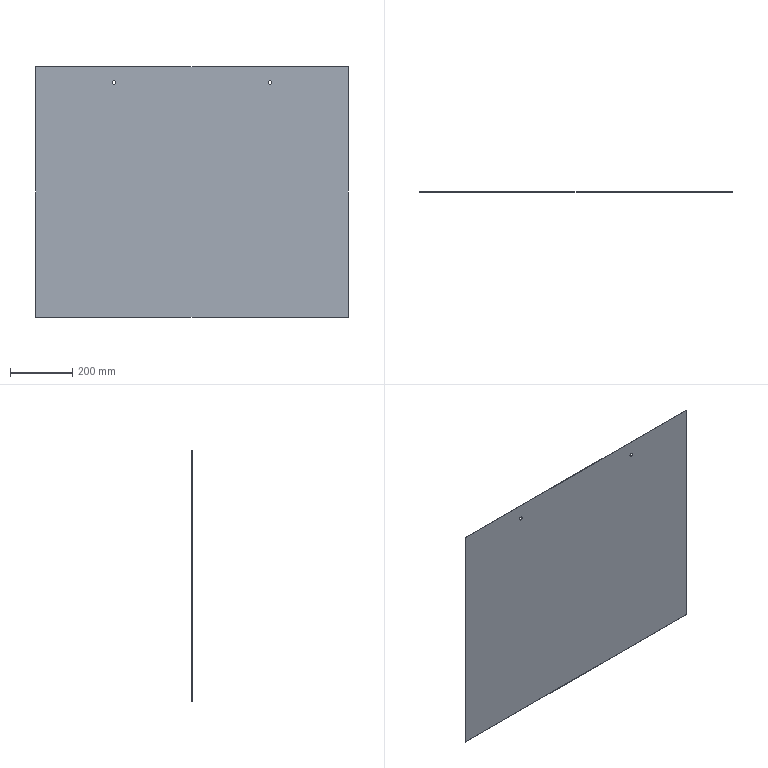Part | SolidWorks | features Extrusion 1, ICE 1 | 1 solid | 10 faces | box 1000 x 1 x 801 mm | volume 800810 mm3 | plane 6 | cylinder 4 | commonest cylinder face diameters 11 x4
STEP:
#1=CARTESIAN_POINT('',(-250.,0.,345.));
#2=VERTEX_POINT('',#1);
#3=CARTESIAN_POINT('',(-250.,0.,356.));
#4=VERTEX_POINT('',#3);
#5=CARTESIAN_POINT('',(-250.,0.,350.5));
#6=DIRECTION('',(0.,1.,0.));
#7=DIRECTION('',(0.,0.,1.));
#8=AXIS2_PLACEMENT_3D('',#5,#6,#7);
#9=CIRCLE('',#8,5.5);
#10=EDGE_CURVE('',#2,#4,#9,.T.);
#11=ORIENTED_EDGE('',*,*,#10,.F.);
#12=CARTESIAN_POINT('',(-250.,1.,345.));
#13=VERTEX_POINT('',#12);
#14=CARTESIAN_POINT('',(-250.,0.,345.));
#15=DIRECTION('',(0.,1.,0.));
#16=VECTOR('',#15,1000.);
#17=LINE('',#14,#16);
#18=EDGE_CURVE('',#2,#13,#17,.T.);
#19=ORIENTED_EDGE('',*,*,#18,.T.);
#20=CARTESIAN_POINT('',(-250.,1.,356.));
#21=VERTEX_POINT('',#20);
#22=CARTESIAN_POINT('',(-250.,1.,350.5));
#23=DIRECTION('',(0.,1.,0.));
#24=DIRECTION('',(0.,0.,1.));
#25=AXIS2_PLACEMENT_3D('',#22,#23,#24);
#26=CIRCLE('',#25,5.5);
#27=EDGE_CURVE('',#13,#21,#26,.T.);
#28=ORIENTED_EDGE('',*,*,#27,.T.);
#29=CARTESIAN_POINT('',(-250.,0.,356.));
#30=DIRECTION('',(0.,1.,0.));
#31=VECTOR('',#30,1000.);
#32=LINE('',#29,#31);
#33=EDGE_CURVE('',#4,#21,#32,.T.);
#34=ORIENTED_EDGE('',*,*,#33,.F.);
#35=EDGE_LOOP('',(#11,#19,#28,#34));
#36=FACE_OUTER_BOUND('',#35,.T.);
#37=CARTESIAN_POINT('',(-250.,0.,350.5));
#38=DIRECTION('',(0.,1.,0.));
#39=DIRECTION('',(0.,0.,1.));
#40=AXIS2_PLACEMENT_3D('',#37,#38,#39);
#41=CYLINDRICAL_SURFACE('',#40,5.5);
#42=ADVANCED_FACE('',(#36),#41,.F.);
#43=CARTESIAN_POINT('',(250.,0.,345.));
#44=VERTEX_POINT('',#43);
#45=CARTESIAN_POINT('',(250.,0.,356.));
#46=VERTEX_POINT('',#45);
#47=CARTESIAN_POINT('',(250.,0.,350.5));
#48=DIRECTION('',(0.,1.,0.));
#49=DIRECTION('',(0.,0.,1.));
#50=AXIS2_PLACEMENT_3D('',#47,#48,#49);
#51=CIRCLE('',#50,5.5);
#52=EDGE_CURVE('',#44,#46,#51,.T.);
#53=ORIENTED_EDGE('',*,*,#52,.F.);
#54=CARTESIAN_POINT('',(250.,1.,345.));
#55=VERTEX_POINT('',#54);
#56=CARTESIAN_POINT('',(250.,0.,345.));
#57=DIRECTION('',(0.,1.,0.));
#58=VECTOR('',#57,1000.);
#59=LINE('',#56,#58);
#60=EDGE_CURVE('',#44,#55,#59,.T.);
#61=ORIENTED_EDGE('',*,*,#60,.T.);
#62=CARTESIAN_POINT('',(250.,1.,356.));
#63=VERTEX_POINT('',#62);
#64=CARTESIAN_POINT('',(250.,1.,350.5));
#65=DIRECTION('',(0.,1.,0.));
#66=DIRECTION('',(0.,0.,1.));
#67=AXIS2_PLACEMENT_3D('',#64,#65,#66);
#68=CIRCLE('',#67,5.5);
#69=EDGE_CURVE('',#55,#63,#68,.T.);
#70=ORIENTED_EDGE('',*,*,#69,.T.);
#71=CARTESIAN_POINT('',(250.,0.,356.));
#72=DIRECTION('',(0.,1.,0.));
#73=VECTOR('',#72,1000.);
#74=LINE('',#71,#73);
#75=EDGE_CURVE('',#46,#63,#74,.T.);
#76=ORIENTED_EDGE('',*,*,#75,.F.);
#77=EDGE_LOOP('',(#53,#61,#70,#76));
#78=FACE_OUTER_BOUND('',#77,.T.);
#79=CARTESIAN_POINT('',(250.,0.,350.5));
#80=DIRECTION('',(0.,1.,0.));
#81=DIRECTION('',(0.,0.,1.));
#82=AXIS2_PLACEMENT_3D('',#79,#80,#81);
#83=CYLINDRICAL_SURFACE('',#82,5.5);
#84=ADVANCED_FACE('',(#78),#83,.F.);
#85=CARTESIAN_POINT('',(500.,0.,400.5));
#86=VERTEX_POINT('',#85);
#87=CARTESIAN_POINT('',(500.,0.,-400.5));
#88=VERTEX_POINT('',#87);
#89=CARTESIAN_POINT('',(500.,0.,400.5));
#90=DIRECTION('',(0.,0.,-1.));
#91=VECTOR('',#90,1000.);
#92=LINE('',#89,#91);
#93=EDGE_CURVE('',#86,#88,#92,.T.);
#94=ORIENTED_EDGE('',*,*,#93,.T.);
#95=CARTESIAN_POINT('',(500.,1.,-400.5));
#96=VERTEX_POINT('',#95);
#97=CARTESIAN_POINT('',(500.,1.,-400.5));
#98=DIRECTION('',(0.,-1.,0.));
#99=VECTOR('',#98,1000.);
#100=LINE('',#97,#99);
#101=EDGE_CURVE('',#96,#88,#100,.T.);
#102=ORIENTED_EDGE('',*,*,#101,.F.);
#103=CARTESIAN_POINT('',(500.,1.,400.5));
#104=VERTEX_POINT('',#103);
#105=CARTESIAN_POINT('',(500.,1.,400.5));
#106=DIRECTION('',(0.,0.,-1.));
#107=VECTOR('',#106,1000.);
#108=LINE('',#105,#107);
#109=EDGE_CURVE('',#104,#96,#108,.T.);
#110=ORIENTED_EDGE('',*,*,#109,.F.);
#111=CARTESIAN_POINT('',(500.,1.,400.5));
#112=DIRECTION('',(0.,-1.,0.));
#113=VECTOR('',#112,1000.);
#114=LINE('',#111,#113);
#115=EDGE_CURVE('',#104,#86,#114,.T.);
#116=ORIENTED_EDGE('',*,*,#115,.T.);
#117=EDGE_LOOP('',(#94,#102,#110,#116));
#118=FACE_OUTER_BOUND('',#117,.T.);
#119=CARTESIAN_POINT('',(500.,1.,400.5));
#120=DIRECTION('',(-1.,0.,0.));
#121=DIRECTION('',(0.,0.,1.));
#122=AXIS2_PLACEMENT_3D('',#119,#120,#121);
#123=PLANE('',#122);
#124=ADVANCED_FACE('',(#118),#123,.F.);
#125=CARTESIAN_POINT('',(-500.,0.,-400.5));
#126=VERTEX_POINT('',#125);
#127=CARTESIAN_POINT('',(-500.,0.,-400.5));
#128=DIRECTION('',(-1.,0.,0.));
#129=VECTOR('',#128,1000.);
#130=LINE('',#127,#129);
#131=EDGE_CURVE('',#88,#126,#130,.T.);
#132=ORIENTED_EDGE('',*,*,#131,.T.);
#133=CARTESIAN_POINT('',(-500.,1.,-400.5));
#134=VERTEX_POINT('',#133);
#135=CARTESIAN_POINT('',(-500.,1.,-400.5));
#136=DIRECTION('',(0.,-1.,0.));
#137=VECTOR('',#136,1000.);
#138=LINE('',#135,#137);
#139=EDGE_CURVE('',#134,#126,#138,.T.);
#140=ORIENTED_EDGE('',*,*,#139,.F.);
#141=CARTESIAN_POINT('',(-500.,1.,-400.5));
#142=DIRECTION('',(-1.,0.,0.));
#143=VECTOR('',#142,1000.);
#144=LINE('',#141,#143);
#145=EDGE_CURVE('',#96,#134,#144,.T.);
#146=ORIENTED_EDGE('',*,*,#145,.F.);
#147=ORIENTED_EDGE('',*,*,#101,.T.);
#148=EDGE_LOOP('',(#132,#140,#146,#147));
#149=FACE_OUTER_BOUND('',#148,.T.);
#150=CARTESIAN_POINT('',(-500.,1.,-400.5));
#151=DIRECTION('',(0.,0.,1.));
#152=DIRECTION('',(1.,0.,0.));
#153=AXIS2_PLACEMENT_3D('',#150,#151,#152);
#154=PLANE('',#153);
#155=ADVANCED_FACE('',(#149),#154,.F.);
#156=CARTESIAN_POINT('',(-500.,0.,400.5));
#157=VERTEX_POINT('',#156);
#158=CARTESIAN_POINT('',(-500.,0.,400.5));
#159=DIRECTION('',(0.,0.,1.));
#160=VECTOR('',#159,1000.);
#161=LINE('',#158,#160);
#162=EDGE_CURVE('',#126,#157,#161,.T.);
#163=ORIENTED_EDGE('',*,*,#162,.T.);
#164=CARTESIAN_POINT('',(-500.,1.,400.5));
#165=VERTEX_POINT('',#164);
#166=CARTESIAN_POINT('',(-500.,1.,400.5));
#167=DIRECTION('',(0.,-1.,0.));
#168=VECTOR('',#167,1000.);
#169=LINE('',#166,#168);
#170=EDGE_CURVE('',#165,#157,#169,.T.);
#171=ORIENTED_EDGE('',*,*,#170,.F.);
#172=CARTESIAN_POINT('',(-500.,1.,400.5));
#173=DIRECTION('',(0.,0.,1.));
#174=VECTOR('',#173,1000.);
#175=LINE('',#172,#174);
#176=EDGE_CURVE('',#134,#165,#175,.T.);
#177=ORIENTED_EDGE('',*,*,#176,.F.);
#178=ORIENTED_EDGE('',*,*,#139,.T.);
#179=EDGE_LOOP('',(#163,#171,#177,#178));
#180=FACE_OUTER_BOUND('',#179,.T.);
#181=CARTESIAN_POINT('',(-500.,1.,400.5));
#182=DIRECTION('',(1.,0.,0.));
#183=DIRECTION('',(0.,0.,-1.));
#184=AXIS2_PLACEMENT_3D('',#181,#182,#183);
#185=PLANE('',#184);
#186=ADVANCED_FACE('',(#180),#185,.F.);
#187=CARTESIAN_POINT('',(-500.,0.,400.5));
#188=DIRECTION('',(1.,0.,0.));
#189=VECTOR('',#188,1000.);
#190=LINE('',#187,#189);
#191=EDGE_CURVE('',#157,#86,#190,.T.);
#192=ORIENTED_EDGE('',*,*,#191,.T.);
#193=ORIENTED_EDGE('',*,*,#115,.F.);
#194=CARTESIAN_POINT('',(-500.,1.,400.5));
#195=DIRECTION('',(1.,0.,0.));
#196=VECTOR('',#195,1000.);
#197=LINE('',#194,#196);
#198=EDGE_CURVE('',#165,#104,#197,.T.);
#199=ORIENTED_EDGE('',*,*,#198,.F.);
#200=ORIENTED_EDGE('',*,*,#170,.T.);
#201=EDGE_LOOP('',(#192,#193,#199,#200));
#202=FACE_OUTER_BOUND('',#201,.T.);
#203=CARTESIAN_POINT('',(-500.,1.,400.5));
#204=DIRECTION('',(0.,0.,-1.));
#205=DIRECTION('',(-1.,0.,0.));
#206=AXIS2_PLACEMENT_3D('',#203,#204,#205);
#207=PLANE('',#206);
#208=ADVANCED_FACE('',(#202),#207,.F.);
#209=CARTESIAN_POINT('',(-250.,1.,350.5));
#210=DIRECTION('',(0.,1.,0.));
#211=DIRECTION('',(0.,0.,1.));
#212=AXIS2_PLACEMENT_3D('',#209,#210,#211);
#213=CIRCLE('',#212,5.5);
#214=EDGE_CURVE('',#21,#13,#213,.T.);
#215=ORIENTED_EDGE('',*,*,#214,.F.);
#216=ORIENTED_EDGE('',*,*,#27,.F.);
#217=EDGE_LOOP('',(#215,#216));
#218=FACE_BOUND('',#217,.T.);
#219=CARTESIAN_POINT('',(250.,1.,350.5));
#220=DIRECTION('',(0.,1.,0.));
#221=DIRECTION('',(0.,0.,1.));
#222=AXIS2_PLACEMENT_3D('',#219,#220,#221);
#223=CIRCLE('',#222,5.5);
#224=EDGE_CURVE('',#63,#55,#223,.T.);
#225=ORIENTED_EDGE('',*,*,#224,.F.);
#226=ORIENTED_EDGE('',*,*,#69,.F.);
#227=EDGE_LOOP('',(#225,#226));
#228=FACE_BOUND('',#227,.T.);
#229=ORIENTED_EDGE('',*,*,#109,.T.);
#230=ORIENTED_EDGE('',*,*,#145,.T.);
#231=ORIENTED_EDGE('',*,*,#176,.T.);
#232=ORIENTED_EDGE('',*,*,#198,.T.);
#233=EDGE_LOOP('',(#229,#230,#231,#232));
#234=FACE_OUTER_BOUND('',#233,.T.);
#235=CARTESIAN_POINT('',(0.,1.,0.));
#236=DIRECTION('',(0.,-1.,0.));
#237=DIRECTION('',(0.,0.,-1.));
#238=AXIS2_PLACEMENT_3D('',#235,#236,#237);
#239=PLANE('',#238);
#240=ADVANCED_FACE('',(#218,#228,#234),#239,.F.);
#241=CARTESIAN_POINT('',(-250.,0.,350.5));
#242=DIRECTION('',(0.,1.,0.));
#243=DIRECTION('',(0.,0.,1.));
#244=AXIS2_PLACEMENT_3D('',#241,#242,#243);
#245=CIRCLE('',#244,5.5);
#246=EDGE_CURVE('',#4,#2,#245,.T.);
#247=ORIENTED_EDGE('',*,*,#246,.T.);
#248=ORIENTED_EDGE('',*,*,#10,.T.);
#249=EDGE_LOOP('',(#247,#248));
#250=FACE_BOUND('',#249,.T.);
#251=CARTESIAN_POINT('',(250.,0.,350.5));
#252=DIRECTION('',(0.,1.,0.));
#253=DIRECTION('',(0.,0.,1.));
#254=AXIS2_PLACEMENT_3D('',#251,#252,#253);
#255=CIRCLE('',#254,5.5);
#256=EDGE_CURVE('',#46,#44,#255,.T.);
#257=ORIENTED_EDGE('',*,*,#256,.T.);
#258=ORIENTED_EDGE('',*,*,#52,.T.);
#259=EDGE_LOOP('',(#257,#258));
#260=FACE_BOUND('',#259,.T.);
#261=ORIENTED_EDGE('',*,*,#93,.F.);
#262=ORIENTED_EDGE('',*,*,#191,.F.);
#263=ORIENTED_EDGE('',*,*,#162,.F.);
#264=ORIENTED_EDGE('',*,*,#131,.F.);
#265=EDGE_LOOP('',(#261,#262,#263,#264));
#266=FACE_OUTER_BOUND('',#265,.T.);
#267=CARTESIAN_POINT('',(0.,0.,0.));
#268=DIRECTION('',(0.,-1.,0.));
#269=DIRECTION('',(0.,0.,-1.));
#270=AXIS2_PLACEMENT_3D('',#267,#268,#269);
#271=PLANE('',#270);
#272=ADVANCED_FACE('',(#250,#260,#266),#271,.T.);
#273=ORIENTED_EDGE('',*,*,#60,.F.);
#274=ORIENTED_EDGE('',*,*,#256,.F.);
#275=ORIENTED_EDGE('',*,*,#75,.T.);
#276=ORIENTED_EDGE('',*,*,#224,.T.);
#277=EDGE_LOOP('',(#273,#274,#275,#276));
#278=FACE_OUTER_BOUND('',#277,.T.);
#279=CARTESIAN_POINT('',(250.,0.,350.5));
#280=DIRECTION('',(0.,1.,0.));
#281=DIRECTION('',(0.,0.,1.));
#282=AXIS2_PLACEMENT_3D('',#279,#280,#281);
#283=CYLINDRICAL_SURFACE('',#282,5.5);
#284=ADVANCED_FACE('',(#278),#283,.F.);
#285=ORIENTED_EDGE('',*,*,#18,.F.);
#286=ORIENTED_EDGE('',*,*,#246,.F.);
#287=ORIENTED_EDGE('',*,*,#33,.T.);
#288=ORIENTED_EDGE('',*,*,#214,.T.);
#289=EDGE_LOOP('',(#285,#286,#287,#288));
#290=FACE_OUTER_BOUND('',#289,.T.);
#291=CARTESIAN_POINT('',(-250.,0.,350.5));
#292=DIRECTION('',(0.,1.,0.));
#293=DIRECTION('',(0.,0.,1.));
#294=AXIS2_PLACEMENT_3D('',#291,#292,#293);
#295=CYLINDRICAL_SURFACE('',#294,5.5);
#296=ADVANCED_FACE('',(#290),#295,.F.);
#297=CLOSED_SHELL('',(#42,#84,#124,#155,#186,#208,#240,#272,#284,#296));
#298=MANIFOLD_SOLID_BREP('',#297);
#299=CARTESIAN_POINT('',(0.,0.,0.));
#300=DIRECTION('',(0.,0.,1.));
#301=DIRECTION('',(1.,0.,0.));
#302=AXIS2_PLACEMENT_3D('',#299,#300,#301);
#303=(LENGTH_UNIT()NAMED_UNIT(*)SI_UNIT(.MILLI.,.METRE.));
#304=UNCERTAINTY_MEASURE_WITH_UNIT(LENGTH_MEASURE(0.00001),#303,'','');
#305=(NAMED_UNIT(*)PLANE_ANGLE_UNIT()SI_UNIT($,.RADIAN.));
#306=(NAMED_UNIT(*)SI_UNIT($,.STERADIAN.)SOLID_ANGLE_UNIT());
#307=(GEOMETRIC_REPRESENTATION_CONTEXT(3)GLOBAL_UNCERTAINTY_ASSIGNED_CONTEXT((#304))GLOBAL_UNIT_ASSIGNED_CONTEXT((#303,#305,#306))REPRESENTATION_CONTEXT('',''));
#308=ADVANCED_BREP_SHAPE_REPRESENTATION('',(#298,#302),#307);